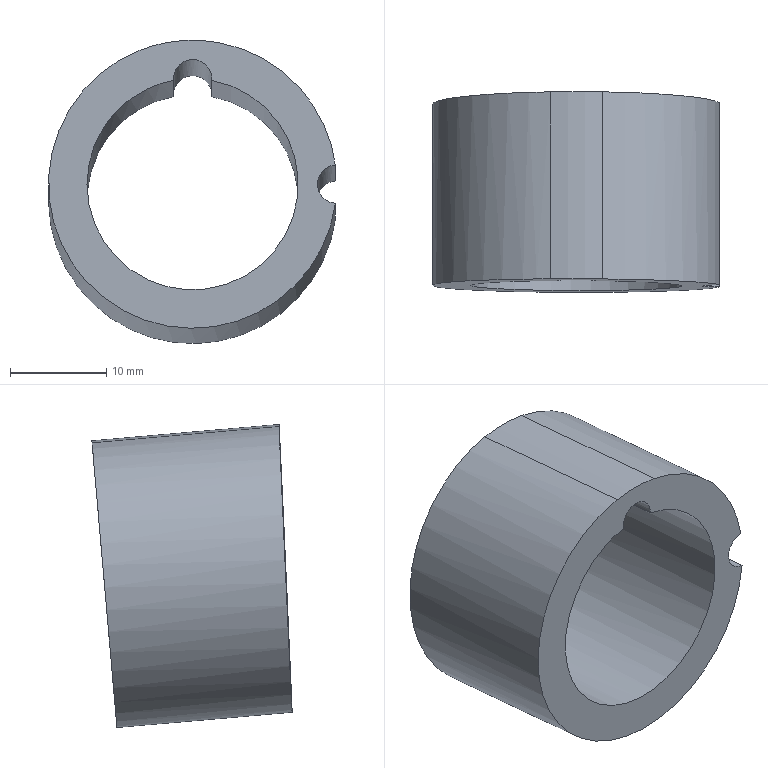Part | NX | features solid 2 | 1 solid | 8 faces | box 29.867 x 20.856 x 31.591 mm | volume 5945 mm3 | cylinder 5 | plane 2 | spline 1 | commonest cylinder face diameters 4 x2 30 x2 22 x1
STEP:
#1=CARTESIAN_POINT('',(121.652,-45.609,-23.587));
#2=VERTEX_POINT('',#1);
#3=CARTESIAN_POINT('',(133.803,-46.213,-36.339));
#4=VERTEX_POINT('',#3);
#5=CARTESIAN_POINT('',(118.936,-46.275,-38.337));
#6=DIRECTION('',(0.001957,0.999,-0.04546));
#7=DIRECTION('',(0.04675,0.04532,0.9979));
#8=AXIS2_PLACEMENT_3D('',#5,#6,#7);
#9=ELLIPSE('',#8,15.013,15.);
#10=EDGE_CURVE('',#2,#4,#9,.T.);
#11=ORIENTED_EDGE('',*,*,#10,.T.);
#12=CARTESIAN_POINT('',(133.803,-27.236,-37.999));
#13=VERTEX_POINT('',#12);
#14=CARTESIAN_POINT('',(133.803,-36.782,-37.164));
#15=DIRECTION('',(0.,0.9962,-0.08716));
#16=VECTOR('',#15,1000.);
#17=LINE('',#14,#16);
#18=EDGE_CURVE('',#4,#13,#17,.T.);
#19=ORIENTED_EDGE('',*,*,#18,.T.);
#20=CARTESIAN_POINT('',(121.652,-26.124,-25.291));
#21=VERTEX_POINT('',#20);
#22=CARTESIAN_POINT('',(118.936,-27.41,-39.987));
#23=DIRECTION('',(0.,0.9962,-0.08716));
#24=DIRECTION('',(0.,0.08716,0.9962));
#25=AXIS2_PLACEMENT_3D('',#22,#23,#24);
#26=CIRCLE('',#25,15.);
#27=EDGE_CURVE('',#21,#13,#26,.T.);
#28=ORIENTED_EDGE('',*,*,#27,.F.);
#29=CARTESIAN_POINT('',(121.652,-26.124,-25.291));
#30=DIRECTION('',(0.,-0.9962,0.08716));
#31=VECTOR('',#30,1000.);
#32=LINE('',#29,#31);
#33=EDGE_CURVE('',#21,#2,#32,.T.);
#34=ORIENTED_EDGE('',*,*,#33,.T.);
#35=EDGE_LOOP('',(#11,#19,#28,#34));
#36=FACE_BOUND('',#35,.T.);
#37=CARTESIAN_POINT('',(118.936,-27.41,-39.987));
#38=DIRECTION('',(0.,-0.9962,0.08716));
#39=DIRECTION('',(0.,-0.08716,-0.9962));
#40=AXIS2_PLACEMENT_3D('',#37,#38,#39);
#41=CYLINDRICAL_SURFACE('',#40,15.);
#42=ADVANCED_FACE('',(#36),#41,.T.);
#43=CARTESIAN_POINT('',(120.928,-45.786,-27.52));
#44=VERTEX_POINT('',#43);
#45=CARTESIAN_POINT('',(116.945,-45.779,-27.521));
#46=VERTEX_POINT('',#45);
#47=CARTESIAN_POINT('',(118.936,-46.275,-38.337));
#48=DIRECTION('',(0.001957,0.999,-0.04546));
#49=DIRECTION('',(0.04675,0.04532,0.9979));
#50=AXIS2_PLACEMENT_3D('',#47,#48,#49);
#51=ELLIPSE('',#50,11.01,11.);
#52=EDGE_CURVE('',#44,#46,#51,.T.);
#53=ORIENTED_EDGE('',*,*,#52,.F.);
#54=CARTESIAN_POINT('',(120.928,-26.467,-29.21));
#55=VERTEX_POINT('',#54);
#56=CARTESIAN_POINT('',(120.928,-26.467,-29.21));
#57=DIRECTION('',(0.,-0.9962,0.08716));
#58=VECTOR('',#57,1000.);
#59=LINE('',#56,#58);
#60=EDGE_CURVE('',#44,#55,#59,.F.);
#61=ORIENTED_EDGE('',*,*,#60,.T.);
#62=CARTESIAN_POINT('',(116.945,-26.467,-29.21));
#63=VERTEX_POINT('',#62);
#64=CARTESIAN_POINT('',(118.936,-27.41,-39.987));
#65=DIRECTION('',(0.,-0.9962,0.08716));
#66=DIRECTION('',(0.,-0.08716,-0.9962));
#67=AXIS2_PLACEMENT_3D('',#64,#65,#66);
#68=CIRCLE('',#67,11.);
#69=EDGE_CURVE('',#55,#63,#68,.F.);
#70=ORIENTED_EDGE('',*,*,#69,.T.);
#71=CARTESIAN_POINT('',(116.945,-26.467,-29.21));
#72=DIRECTION('',(0.,-0.9962,0.08716));
#73=VECTOR('',#72,1000.);
#74=LINE('',#71,#73);
#75=EDGE_CURVE('',#63,#46,#74,.T.);
#76=ORIENTED_EDGE('',*,*,#75,.T.);
#77=EDGE_LOOP('',(#53,#61,#70,#76));
#78=FACE_BOUND('',#77,.T.);
#79=CARTESIAN_POINT('',(118.936,-27.41,-39.987));
#80=DIRECTION('',(0.,-0.9962,0.08716));
#81=DIRECTION('',(0.,-0.08716,-0.9962));
#82=AXIS2_PLACEMENT_3D('',#79,#80,#81);
#83=CYLINDRICAL_SURFACE('',#82,11.);
#84=ADVANCED_FACE('',(#78),#83,.F.);
#85=CARTESIAN_POINT('',(118.936,-26.451,-29.029));
#86=DIRECTION('',(0.,-0.9962,0.08716));
#87=DIRECTION('',(0.,-0.08716,-0.9962));
#88=AXIS2_PLACEMENT_3D('',#85,#86,#87);
#89=CIRCLE('',#88,2.);
#90=EDGE_CURVE('',#55,#63,#89,.T.);
#91=ORIENTED_EDGE('',*,*,#90,.T.);
#92=ORIENTED_EDGE('',*,*,#69,.F.);
#93=EDGE_LOOP('',(#91,#92));
#94=FACE_BOUND('',#93,.T.);
#95=CARTESIAN_POINT('',(133.803,-27.583,-41.975));
#96=VERTEX_POINT('',#95);
#97=CARTESIAN_POINT('',(133.936,-27.41,-39.987));
#98=DIRECTION('',(0.,-0.9962,0.08716));
#99=DIRECTION('',(0.,-0.08716,-0.9962));
#100=AXIS2_PLACEMENT_3D('',#97,#98,#99);
#101=CIRCLE('',#100,2.);
#102=EDGE_CURVE('',#13,#96,#101,.T.);
#103=ORIENTED_EDGE('',*,*,#102,.T.);
#104=CARTESIAN_POINT('',(116.22,-26.124,-25.291));
#105=VERTEX_POINT('',#104);
#106=CARTESIAN_POINT('',(118.936,-27.41,-39.987));
#107=DIRECTION('',(0.,0.9962,-0.08716));
#108=DIRECTION('',(0.,0.08716,0.9962));
#109=AXIS2_PLACEMENT_3D('',#106,#107,#108);
#110=CIRCLE('',#109,15.);
#111=EDGE_CURVE('',#96,#105,#110,.T.);
#112=ORIENTED_EDGE('',*,*,#111,.T.);
#113=CARTESIAN_POINT('',(116.22,-26.124,-25.291));
#114=CARTESIAN_POINT('',(118.016,-26.095,-24.962));
#115=CARTESIAN_POINT('',(119.857,-26.095,-24.962));
#116=CARTESIAN_POINT('',(121.652,-26.124,-25.291));
#117=B_SPLINE_CURVE_WITH_KNOTS('',3,(#113,#114,#115,#116),.UNSPECIFIED.,.F.,.F.,(4,4),(0.,1.),.PIECEWISE_BEZIER_KNOTS.);
#118=EDGE_CURVE('',#105,#21,#117,.T.);
#119=ORIENTED_EDGE('',*,*,#118,.T.);
#120=ORIENTED_EDGE('',*,*,#27,.T.);
#121=EDGE_LOOP('',(#103,#112,#119,#120));
#122=FACE_BOUND('',#121,.T.);
#123=CARTESIAN_POINT('',(116.22,-26.124,-25.291));
#124=DIRECTION('',(0.,0.9962,-0.08716));
#125=DIRECTION('',(0.,0.08716,0.9962));
#126=AXIS2_PLACEMENT_3D('',#123,#124,#125);
#127=PLANE('',#126);
#128=ADVANCED_FACE('',(#94,#122),#127,.T.);
#129=CARTESIAN_POINT('',(118.936,-45.774,-27.338));
#130=DIRECTION('',(0.001957,0.999,-0.04546));
#131=DIRECTION('',(-0.04675,-0.04532,-0.9979));
#132=AXIS2_PLACEMENT_3D('',#129,#130,#131);
#133=ELLIPSE('',#132,2.002,2.);
#134=EDGE_CURVE('',#46,#44,#133,.T.);
#135=ORIENTED_EDGE('',*,*,#134,.T.);
#136=ORIENTED_EDGE('',*,*,#52,.T.);
#137=EDGE_LOOP('',(#135,#136));
#138=FACE_BOUND('',#137,.T.);
#139=CARTESIAN_POINT('',(133.803,-46.395,-40.329));
#140=VERTEX_POINT('',#139);
#141=CARTESIAN_POINT('',(133.936,-46.304,-38.334));
#142=DIRECTION('',(0.001957,0.999,-0.04546));
#143=DIRECTION('',(-0.04675,-0.04532,-0.9979));
#144=AXIS2_PLACEMENT_3D('',#141,#142,#143);
#145=ELLIPSE('',#144,2.002,2.);
#146=EDGE_CURVE('',#140,#4,#145,.T.);
#147=ORIENTED_EDGE('',*,*,#146,.T.);
#148=ORIENTED_EDGE('',*,*,#10,.F.);
#149=CARTESIAN_POINT('',(116.22,-45.598,-23.587));
#150=VERTEX_POINT('',#149);
#151=CARTESIAN_POINT('',(116.22,-45.598,-23.587));
#152=CARTESIAN_POINT('',(118.014,-45.587,-23.257));
#153=CARTESIAN_POINT('',(119.859,-45.59,-23.257));
#154=CARTESIAN_POINT('',(121.652,-45.609,-23.587));
#155=B_SPLINE_CURVE_WITH_KNOTS('',3,(#151,#152,#153,#154),.UNSPECIFIED.,.F.,.F.,(4,4),(0.,0.005466),.UNSPECIFIED.);
#156=EDGE_CURVE('',#150,#2,#155,.T.);
#157=ORIENTED_EDGE('',*,*,#156,.F.);
#158=CARTESIAN_POINT('',(118.936,-46.275,-38.337));
#159=DIRECTION('',(0.001957,0.999,-0.04546));
#160=DIRECTION('',(0.04675,0.04532,0.9979));
#161=AXIS2_PLACEMENT_3D('',#158,#159,#160);
#162=ELLIPSE('',#161,15.013,15.);
#163=EDGE_CURVE('',#140,#150,#162,.T.);
#164=ORIENTED_EDGE('',*,*,#163,.F.);
#165=EDGE_LOOP('',(#147,#148,#157,#164));
#166=FACE_BOUND('',#165,.T.);
#167=CARTESIAN_POINT('',(128.811,-48.589,-88.763));
#168=DIRECTION('',(0.001957,0.999,-0.04546));
#169=DIRECTION('',(0.06617,0.04523,0.9968));
#170=AXIS2_PLACEMENT_3D('',#167,#168,#169);
#171=PLANE('',#170);
#172=ADVANCED_FACE('',(#138,#166),#171,.F.);
#173=ORIENTED_EDGE('',*,*,#111,.F.);
#174=CARTESIAN_POINT('',(133.803,-37.129,-41.14));
#175=DIRECTION('',(0.,0.9962,-0.08716));
#176=VECTOR('',#175,1000.);
#177=LINE('',#174,#176);
#178=EDGE_CURVE('',#96,#140,#177,.F.);
#179=ORIENTED_EDGE('',*,*,#178,.T.);
#180=ORIENTED_EDGE('',*,*,#163,.T.);
#181=CARTESIAN_POINT('',(116.22,-26.124,-25.291));
#182=DIRECTION('',(0.,-0.9962,0.08716));
#183=VECTOR('',#182,1000.);
#184=LINE('',#181,#183);
#185=EDGE_CURVE('',#105,#150,#184,.T.);
#186=ORIENTED_EDGE('',*,*,#185,.F.);
#187=EDGE_LOOP('',(#173,#179,#180,#186));
#188=FACE_BOUND('',#187,.T.);
#189=CARTESIAN_POINT('',(118.936,-27.41,-39.987));
#190=DIRECTION('',(0.,-0.9962,0.08716));
#191=DIRECTION('',(0.,-0.08716,-0.9962));
#192=AXIS2_PLACEMENT_3D('',#189,#190,#191);
#193=CYLINDRICAL_SURFACE('',#192,15.);
#194=ADVANCED_FACE('',(#188),#193,.T.);
#195=ORIENTED_EDGE('',*,*,#156,.T.);
#196=ORIENTED_EDGE('',*,*,#33,.F.);
#197=ORIENTED_EDGE('',*,*,#118,.F.);
#198=ORIENTED_EDGE('',*,*,#185,.T.);
#199=EDGE_LOOP('',(#195,#196,#197,#198));
#200=FACE_BOUND('',#199,.T.);
#201=CARTESIAN_POINT('',(116.22,-26.124,-25.291));
#202=CARTESIAN_POINT('',(116.22,-45.733,-23.576));
#203=CARTESIAN_POINT('',(118.016,-26.095,-24.962));
#204=CARTESIAN_POINT('',(118.016,-45.704,-23.246));
#205=CARTESIAN_POINT('',(119.857,-26.095,-24.962));
#206=CARTESIAN_POINT('',(119.857,-45.704,-23.246));
#207=CARTESIAN_POINT('',(121.652,-26.124,-25.291));
#208=CARTESIAN_POINT('',(121.652,-45.733,-23.576));
#209=B_SPLINE_SURFACE_WITH_KNOTS('',3,1,((#201,#202),(#203,#204),(#205,#206),(#207,#208)),.SURF_OF_LINEAR_EXTRUSION.,.F.,.F.,.F.,(4,4),(2,2),(0.,1.),(0.,1.),.PIECEWISE_BEZIER_KNOTS.);
#210=ADVANCED_FACE('',(#200),#209,.F.);
#211=ORIENTED_EDGE('',*,*,#146,.F.);
#212=ORIENTED_EDGE('',*,*,#178,.F.);
#213=ORIENTED_EDGE('',*,*,#102,.F.);
#214=ORIENTED_EDGE('',*,*,#18,.F.);
#215=EDGE_LOOP('',(#211,#212,#213,#214));
#216=FACE_BOUND('',#215,.T.);
#217=CARTESIAN_POINT('',(133.936,-47.333,-38.244));
#218=DIRECTION('',(0.,0.9962,-0.08716));
#219=DIRECTION('',(0.,0.08716,0.9962));
#220=AXIS2_PLACEMENT_3D('',#217,#218,#219);
#221=CYLINDRICAL_SURFACE('',#220,2.);
#222=ADVANCED_FACE('',(#216),#221,.F.);
#223=ORIENTED_EDGE('',*,*,#75,.F.);
#224=ORIENTED_EDGE('',*,*,#90,.F.);
#225=ORIENTED_EDGE('',*,*,#60,.F.);
#226=ORIENTED_EDGE('',*,*,#134,.F.);
#227=EDGE_LOOP('',(#223,#224,#225,#226));
#228=FACE_BOUND('',#227,.T.);
#229=CARTESIAN_POINT('',(118.936,-46.375,-27.286));
#230=DIRECTION('',(0.,0.9962,-0.08716));
#231=DIRECTION('',(0.,0.08716,0.9962));
#232=AXIS2_PLACEMENT_3D('',#229,#230,#231);
#233=CYLINDRICAL_SURFACE('',#232,2.);
#234=ADVANCED_FACE('',(#228),#233,.F.);
#235=CLOSED_SHELL('',(#42,#84,#128,#172,#194,#210,#222,#234));
#236=MANIFOLD_SOLID_BREP('',#235);
#237=(LENGTH_UNIT()NAMED_UNIT(*)SI_UNIT(.MILLI.,.METRE.));
#238=UNCERTAINTY_MEASURE_WITH_UNIT(LENGTH_MEASURE(0.0508),#237,'','');
#239=(NAMED_UNIT(*)PLANE_ANGLE_UNIT()SI_UNIT($,.RADIAN.));
#240=(NAMED_UNIT(*)SI_UNIT($,.STERADIAN.)SOLID_ANGLE_UNIT());
#241=(GEOMETRIC_REPRESENTATION_CONTEXT(3)GLOBAL_UNCERTAINTY_ASSIGNED_CONTEXT((#238))GLOBAL_UNIT_ASSIGNED_CONTEXT((#237,#239,#240))REPRESENTATION_CONTEXT('',''));
#242=ADVANCED_BREP_SHAPE_REPRESENTATION('',(#236),#241);